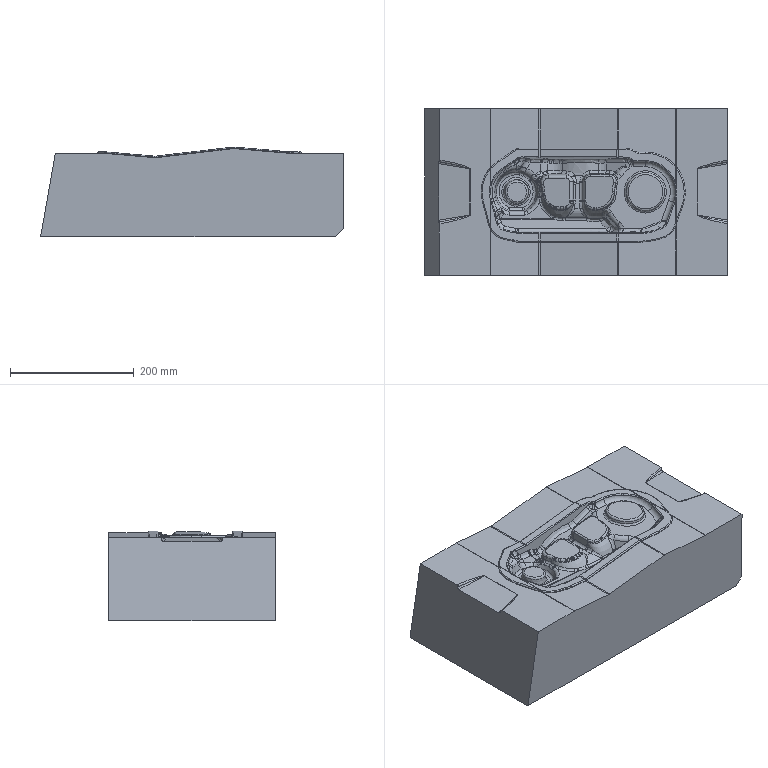Part | 1 solid | 495 faces | box 490.523 x 270 x 145.452 mm | volume 17185915 mm3 | spline 326 | cylinder 65 | plane 54 | torus 32 | cone 13 | sphere 5 | commonest cylinder face diameters 3.4 x17 20 x12 10.15 x6 6 x4 12.18 x4 15 x4